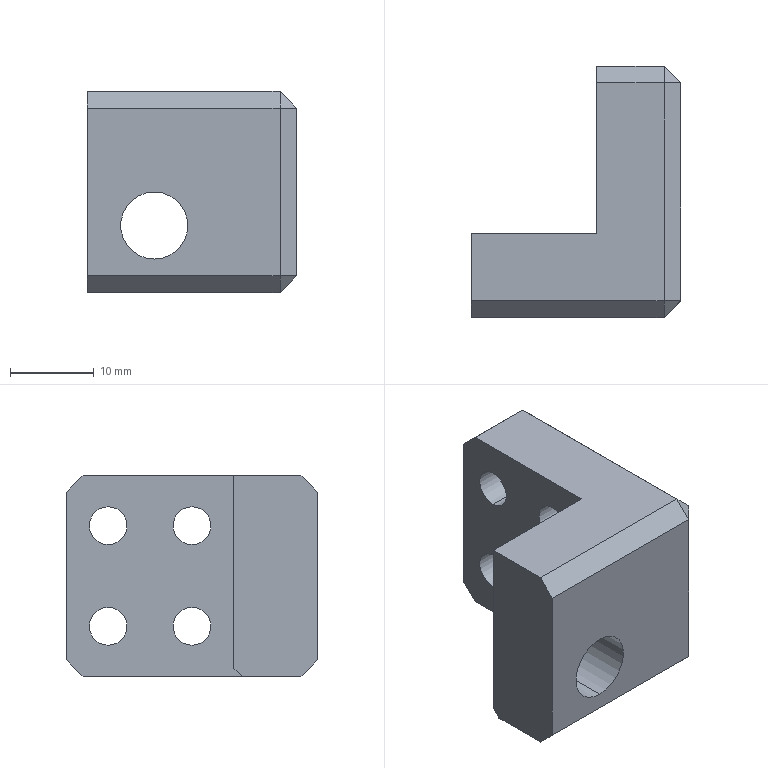Part | NX | features BREP 1 | 1 solid | 45 faces | box 25 x 30 x 24 mm | volume 8772 mm3 | plane 27 | cylinder 18 | commonest cylinder face diameters 8 x10 4.5 x8
STEP:
#1=CARTESIAN_POINT('',(3.971,-310.,10.));
#2=VERTEX_POINT('',#1);
#3=CARTESIAN_POINT('',(3.971,-310.,2.));
#4=VERTEX_POINT('',#3);
#5=CARTESIAN_POINT('',(3.971,-310.,6.));
#6=DIRECTION('',(1.,0.,0.));
#7=DIRECTION('',(0.,0.,-1.));
#8=AXIS2_PLACEMENT_3D('',#5,#6,#7);
#9=CIRCLE('',#8,4.);
#10=EDGE_CURVE('',#2,#4,#9,.T.);
#11=ORIENTED_EDGE('',*,*,#10,.F.);
#12=CARTESIAN_POINT('',(7.971,-310.,10.));
#13=VERTEX_POINT('',#12);
#14=CARTESIAN_POINT('',(7.971,-310.,10.));
#15=DIRECTION('',(1.,0.,0.));
#16=VECTOR('',#15,1000.);
#17=LINE('',#14,#16);
#18=EDGE_CURVE('',#2,#13,#17,.T.);
#19=ORIENTED_EDGE('',*,*,#18,.T.);
#20=CARTESIAN_POINT('',(7.971,-310.,2.));
#21=VERTEX_POINT('',#20);
#22=CARTESIAN_POINT('',(7.971,-310.,6.));
#23=DIRECTION('',(1.,0.,0.));
#24=DIRECTION('',(0.,0.,-1.));
#25=AXIS2_PLACEMENT_3D('',#22,#23,#24);
#26=CIRCLE('',#25,4.);
#27=EDGE_CURVE('',#13,#21,#26,.T.);
#28=ORIENTED_EDGE('',*,*,#27,.T.);
#29=CARTESIAN_POINT('',(7.971,-310.,2.));
#30=DIRECTION('',(1.,0.,0.));
#31=VECTOR('',#30,1000.);
#32=LINE('',#29,#31);
#33=EDGE_CURVE('',#4,#21,#32,.T.);
#34=ORIENTED_EDGE('',*,*,#33,.F.);
#35=EDGE_LOOP('',(#11,#19,#28,#34));
#36=FACE_BOUND('',#35,.T.);
#37=CARTESIAN_POINT('',(7.971,-310.,6.));
#38=DIRECTION('',(1.,0.,0.));
#39=DIRECTION('',(0.,0.,-1.));
#40=AXIS2_PLACEMENT_3D('',#37,#38,#39);
#41=CYLINDRICAL_SURFACE('',#40,4.);
#42=ADVANCED_FACE('',(#36),#41,.F.);
#43=CARTESIAN_POINT('',(-2.029,-310.,8.25));
#44=VERTEX_POINT('',#43);
#45=CARTESIAN_POINT('',(-2.029,-310.,3.75));
#46=VERTEX_POINT('',#45);
#47=CARTESIAN_POINT('',(-2.029,-310.,6.));
#48=DIRECTION('',(1.,0.,0.));
#49=DIRECTION('',(0.,1.,0.));
#50=AXIS2_PLACEMENT_3D('',#47,#48,#49);
#51=CIRCLE('',#50,2.25);
#52=EDGE_CURVE('',#44,#46,#51,.T.);
#53=ORIENTED_EDGE('',*,*,#52,.F.);
#54=CARTESIAN_POINT('',(3.971,-310.,8.25));
#55=VERTEX_POINT('',#54);
#56=CARTESIAN_POINT('',(7.971,-310.,8.25));
#57=DIRECTION('',(1.,0.,0.));
#58=VECTOR('',#57,1000.);
#59=LINE('',#56,#58);
#60=EDGE_CURVE('',#44,#55,#59,.T.);
#61=ORIENTED_EDGE('',*,*,#60,.T.);
#62=CARTESIAN_POINT('',(3.971,-310.,3.75));
#63=VERTEX_POINT('',#62);
#64=CARTESIAN_POINT('',(3.971,-310.,6.));
#65=DIRECTION('',(1.,0.,0.));
#66=DIRECTION('',(0.,0.,-1.));
#67=AXIS2_PLACEMENT_3D('',#64,#65,#66);
#68=CIRCLE('',#67,2.25);
#69=EDGE_CURVE('',#55,#63,#68,.T.);
#70=ORIENTED_EDGE('',*,*,#69,.T.);
#71=CARTESIAN_POINT('',(7.971,-310.,3.75));
#72=DIRECTION('',(1.,0.,0.));
#73=VECTOR('',#72,1000.);
#74=LINE('',#71,#73);
#75=EDGE_CURVE('',#46,#63,#74,.T.);
#76=ORIENTED_EDGE('',*,*,#75,.F.);
#77=EDGE_LOOP('',(#53,#61,#70,#76));
#78=FACE_BOUND('',#77,.T.);
#79=CARTESIAN_POINT('',(7.971,-310.,6.));
#80=DIRECTION('',(1.,0.,0.));
#81=DIRECTION('',(0.,0.,-1.));
#82=AXIS2_PLACEMENT_3D('',#79,#80,#81);
#83=CYLINDRICAL_SURFACE('',#82,2.25);
#84=ADVANCED_FACE('',(#78),#83,.F.);
#85=CARTESIAN_POINT('',(3.971,-320.,10.));
#86=VERTEX_POINT('',#85);
#87=CARTESIAN_POINT('',(3.971,-320.,2.));
#88=VERTEX_POINT('',#87);
#89=CARTESIAN_POINT('',(3.971,-320.,6.));
#90=DIRECTION('',(1.,0.,0.));
#91=DIRECTION('',(0.,0.,-1.));
#92=AXIS2_PLACEMENT_3D('',#89,#90,#91);
#93=CIRCLE('',#92,4.);
#94=EDGE_CURVE('',#86,#88,#93,.T.);
#95=ORIENTED_EDGE('',*,*,#94,.F.);
#96=CARTESIAN_POINT('',(7.971,-320.,10.));
#97=VERTEX_POINT('',#96);
#98=CARTESIAN_POINT('',(7.971,-320.,10.));
#99=DIRECTION('',(1.,0.,0.));
#100=VECTOR('',#99,1000.);
#101=LINE('',#98,#100);
#102=EDGE_CURVE('',#86,#97,#101,.T.);
#103=ORIENTED_EDGE('',*,*,#102,.T.);
#104=CARTESIAN_POINT('',(7.971,-320.,2.));
#105=VERTEX_POINT('',#104);
#106=CARTESIAN_POINT('',(7.971,-320.,6.));
#107=DIRECTION('',(1.,0.,0.));
#108=DIRECTION('',(0.,0.,-1.));
#109=AXIS2_PLACEMENT_3D('',#106,#107,#108);
#110=CIRCLE('',#109,4.);
#111=EDGE_CURVE('',#97,#105,#110,.T.);
#112=ORIENTED_EDGE('',*,*,#111,.T.);
#113=CARTESIAN_POINT('',(7.971,-320.,2.));
#114=DIRECTION('',(1.,0.,0.));
#115=VECTOR('',#114,1000.);
#116=LINE('',#113,#115);
#117=EDGE_CURVE('',#88,#105,#116,.T.);
#118=ORIENTED_EDGE('',*,*,#117,.F.);
#119=EDGE_LOOP('',(#95,#103,#112,#118));
#120=FACE_BOUND('',#119,.T.);
#121=CARTESIAN_POINT('',(7.971,-320.,6.));
#122=DIRECTION('',(1.,0.,0.));
#123=DIRECTION('',(0.,0.,-1.));
#124=AXIS2_PLACEMENT_3D('',#121,#122,#123);
#125=CYLINDRICAL_SURFACE('',#124,4.);
#126=ADVANCED_FACE('',(#120),#125,.F.);
#127=CARTESIAN_POINT('',(-2.029,-320.,8.25));
#128=VERTEX_POINT('',#127);
#129=CARTESIAN_POINT('',(-2.029,-320.,3.75));
#130=VERTEX_POINT('',#129);
#131=CARTESIAN_POINT('',(-2.029,-320.,6.));
#132=DIRECTION('',(1.,0.,0.));
#133=DIRECTION('',(0.,1.,0.));
#134=AXIS2_PLACEMENT_3D('',#131,#132,#133);
#135=CIRCLE('',#134,2.25);
#136=EDGE_CURVE('',#128,#130,#135,.T.);
#137=ORIENTED_EDGE('',*,*,#136,.F.);
#138=CARTESIAN_POINT('',(3.971,-320.,8.25));
#139=VERTEX_POINT('',#138);
#140=CARTESIAN_POINT('',(7.971,-320.,8.25));
#141=DIRECTION('',(1.,0.,0.));
#142=VECTOR('',#141,1000.);
#143=LINE('',#140,#142);
#144=EDGE_CURVE('',#128,#139,#143,.T.);
#145=ORIENTED_EDGE('',*,*,#144,.T.);
#146=CARTESIAN_POINT('',(3.971,-320.,3.75));
#147=VERTEX_POINT('',#146);
#148=CARTESIAN_POINT('',(3.971,-320.,6.));
#149=DIRECTION('',(1.,0.,0.));
#150=DIRECTION('',(0.,0.,-1.));
#151=AXIS2_PLACEMENT_3D('',#148,#149,#150);
#152=CIRCLE('',#151,2.25);
#153=EDGE_CURVE('',#139,#147,#152,.T.);
#154=ORIENTED_EDGE('',*,*,#153,.T.);
#155=CARTESIAN_POINT('',(7.971,-320.,3.75));
#156=DIRECTION('',(1.,0.,0.));
#157=VECTOR('',#156,1000.);
#158=LINE('',#155,#157);
#159=EDGE_CURVE('',#130,#147,#158,.T.);
#160=ORIENTED_EDGE('',*,*,#159,.F.);
#161=EDGE_LOOP('',(#137,#145,#154,#160));
#162=FACE_BOUND('',#161,.T.);
#163=CARTESIAN_POINT('',(7.971,-320.,6.));
#164=DIRECTION('',(1.,0.,0.));
#165=DIRECTION('',(0.,0.,-1.));
#166=AXIS2_PLACEMENT_3D('',#163,#164,#165);
#167=CYLINDRICAL_SURFACE('',#166,2.25);
#168=ADVANCED_FACE('',(#162),#167,.F.);
#169=CARTESIAN_POINT('',(3.971,-310.,22.));
#170=VERTEX_POINT('',#169);
#171=CARTESIAN_POINT('',(3.971,-310.,14.));
#172=VERTEX_POINT('',#171);
#173=CARTESIAN_POINT('',(3.971,-310.,18.));
#174=DIRECTION('',(1.,0.,0.));
#175=DIRECTION('',(0.,0.,-1.));
#176=AXIS2_PLACEMENT_3D('',#173,#174,#175);
#177=CIRCLE('',#176,4.);
#178=EDGE_CURVE('',#170,#172,#177,.T.);
#179=ORIENTED_EDGE('',*,*,#178,.F.);
#180=CARTESIAN_POINT('',(7.971,-310.,22.));
#181=VERTEX_POINT('',#180);
#182=CARTESIAN_POINT('',(7.971,-310.,22.));
#183=DIRECTION('',(1.,0.,0.));
#184=VECTOR('',#183,1000.);
#185=LINE('',#182,#184);
#186=EDGE_CURVE('',#170,#181,#185,.T.);
#187=ORIENTED_EDGE('',*,*,#186,.T.);
#188=CARTESIAN_POINT('',(7.971,-310.,14.));
#189=VERTEX_POINT('',#188);
#190=CARTESIAN_POINT('',(7.971,-310.,18.));
#191=DIRECTION('',(1.,0.,0.));
#192=DIRECTION('',(0.,0.,-1.));
#193=AXIS2_PLACEMENT_3D('',#190,#191,#192);
#194=CIRCLE('',#193,4.);
#195=EDGE_CURVE('',#181,#189,#194,.T.);
#196=ORIENTED_EDGE('',*,*,#195,.T.);
#197=CARTESIAN_POINT('',(7.971,-310.,14.));
#198=DIRECTION('',(1.,0.,0.));
#199=VECTOR('',#198,1000.);
#200=LINE('',#197,#199);
#201=EDGE_CURVE('',#172,#189,#200,.T.);
#202=ORIENTED_EDGE('',*,*,#201,.F.);
#203=EDGE_LOOP('',(#179,#187,#196,#202));
#204=FACE_BOUND('',#203,.T.);
#205=CARTESIAN_POINT('',(7.971,-310.,18.));
#206=DIRECTION('',(1.,0.,0.));
#207=DIRECTION('',(0.,0.,-1.));
#208=AXIS2_PLACEMENT_3D('',#205,#206,#207);
#209=CYLINDRICAL_SURFACE('',#208,4.);
#210=ADVANCED_FACE('',(#204),#209,.F.);
#211=CARTESIAN_POINT('',(-2.029,-310.,20.25));
#212=VERTEX_POINT('',#211);
#213=CARTESIAN_POINT('',(-2.029,-310.,15.75));
#214=VERTEX_POINT('',#213);
#215=CARTESIAN_POINT('',(-2.029,-310.,18.));
#216=DIRECTION('',(1.,0.,0.));
#217=DIRECTION('',(0.,1.,0.));
#218=AXIS2_PLACEMENT_3D('',#215,#216,#217);
#219=CIRCLE('',#218,2.25);
#220=EDGE_CURVE('',#212,#214,#219,.T.);
#221=ORIENTED_EDGE('',*,*,#220,.F.);
#222=CARTESIAN_POINT('',(3.971,-310.,20.25));
#223=VERTEX_POINT('',#222);
#224=CARTESIAN_POINT('',(7.971,-310.,20.25));
#225=DIRECTION('',(1.,0.,0.));
#226=VECTOR('',#225,1000.);
#227=LINE('',#224,#226);
#228=EDGE_CURVE('',#212,#223,#227,.T.);
#229=ORIENTED_EDGE('',*,*,#228,.T.);
#230=CARTESIAN_POINT('',(3.971,-310.,15.75));
#231=VERTEX_POINT('',#230);
#232=CARTESIAN_POINT('',(3.971,-310.,18.));
#233=DIRECTION('',(1.,0.,0.));
#234=DIRECTION('',(0.,0.,-1.));
#235=AXIS2_PLACEMENT_3D('',#232,#233,#234);
#236=CIRCLE('',#235,2.25);
#237=EDGE_CURVE('',#223,#231,#236,.T.);
#238=ORIENTED_EDGE('',*,*,#237,.T.);
#239=CARTESIAN_POINT('',(7.971,-310.,15.75));
#240=DIRECTION('',(1.,0.,0.));
#241=VECTOR('',#240,1000.);
#242=LINE('',#239,#241);
#243=EDGE_CURVE('',#214,#231,#242,.T.);
#244=ORIENTED_EDGE('',*,*,#243,.F.);
#245=EDGE_LOOP('',(#221,#229,#238,#244));
#246=FACE_BOUND('',#245,.T.);
#247=CARTESIAN_POINT('',(7.971,-310.,18.));
#248=DIRECTION('',(1.,0.,0.));
#249=DIRECTION('',(0.,0.,-1.));
#250=AXIS2_PLACEMENT_3D('',#247,#248,#249);
#251=CYLINDRICAL_SURFACE('',#250,2.25);
#252=ADVANCED_FACE('',(#246),#251,.F.);
#253=CARTESIAN_POINT('',(3.971,-320.,22.));
#254=VERTEX_POINT('',#253);
#255=CARTESIAN_POINT('',(3.971,-320.,14.));
#256=VERTEX_POINT('',#255);
#257=CARTESIAN_POINT('',(3.971,-320.,18.));
#258=DIRECTION('',(1.,0.,0.));
#259=DIRECTION('',(0.,0.,-1.));
#260=AXIS2_PLACEMENT_3D('',#257,#258,#259);
#261=CIRCLE('',#260,4.);
#262=EDGE_CURVE('',#254,#256,#261,.T.);
#263=ORIENTED_EDGE('',*,*,#262,.F.);
#264=CARTESIAN_POINT('',(7.971,-320.,22.));
#265=VERTEX_POINT('',#264);
#266=CARTESIAN_POINT('',(7.971,-320.,22.));
#267=DIRECTION('',(1.,0.,0.));
#268=VECTOR('',#267,1000.);
#269=LINE('',#266,#268);
#270=EDGE_CURVE('',#254,#265,#269,.T.);
#271=ORIENTED_EDGE('',*,*,#270,.T.);
#272=CARTESIAN_POINT('',(7.971,-320.,14.));
#273=VERTEX_POINT('',#272);
#274=CARTESIAN_POINT('',(7.971,-320.,18.));
#275=DIRECTION('',(1.,0.,0.));
#276=DIRECTION('',(0.,0.,-1.));
#277=AXIS2_PLACEMENT_3D('',#274,#275,#276);
#278=CIRCLE('',#277,4.);
#279=EDGE_CURVE('',#265,#273,#278,.T.);
#280=ORIENTED_EDGE('',*,*,#279,.T.);
#281=CARTESIAN_POINT('',(7.971,-320.,14.));
#282=DIRECTION('',(1.,0.,0.));
#283=VECTOR('',#282,1000.);
#284=LINE('',#281,#283);
#285=EDGE_CURVE('',#256,#273,#284,.T.);
#286=ORIENTED_EDGE('',*,*,#285,.F.);
#287=EDGE_LOOP('',(#263,#271,#280,#286));
#288=FACE_BOUND('',#287,.T.);
#289=CARTESIAN_POINT('',(7.971,-320.,18.));
#290=DIRECTION('',(1.,0.,0.));
#291=DIRECTION('',(0.,0.,-1.));
#292=AXIS2_PLACEMENT_3D('',#289,#290,#291);
#293=CYLINDRICAL_SURFACE('',#292,4.);
#294=ADVANCED_FACE('',(#288),#293,.F.);
#295=CARTESIAN_POINT('',(-2.029,-320.,20.25));
#296=VERTEX_POINT('',#295);
#297=CARTESIAN_POINT('',(-2.029,-320.,15.75));
#298=VERTEX_POINT('',#297);
#299=CARTESIAN_POINT('',(-2.029,-320.,18.));
#300=DIRECTION('',(1.,0.,0.));
#301=DIRECTION('',(0.,1.,0.));
#302=AXIS2_PLACEMENT_3D('',#299,#300,#301);
#303=CIRCLE('',#302,2.25);
#304=EDGE_CURVE('',#296,#298,#303,.T.);
#305=ORIENTED_EDGE('',*,*,#304,.F.);
#306=CARTESIAN_POINT('',(3.971,-320.,20.25));
#307=VERTEX_POINT('',#306);
#308=CARTESIAN_POINT('',(7.971,-320.,20.25));
#309=DIRECTION('',(1.,0.,0.));
#310=VECTOR('',#309,1000.);
#311=LINE('',#308,#310);
#312=EDGE_CURVE('',#296,#307,#311,.T.);
#313=ORIENTED_EDGE('',*,*,#312,.T.);
#314=CARTESIAN_POINT('',(3.971,-320.,15.75));
#315=VERTEX_POINT('',#314);
#316=CARTESIAN_POINT('',(3.971,-320.,18.));
#317=DIRECTION('',(1.,0.,0.));
#318=DIRECTION('',(0.,0.,-1.));
#319=AXIS2_PLACEMENT_3D('',#316,#317,#318);
#320=CIRCLE('',#319,2.25);
#321=EDGE_CURVE('',#307,#315,#320,.T.);
#322=ORIENTED_EDGE('',*,*,#321,.T.);
#323=CARTESIAN_POINT('',(7.971,-320.,15.75));
#324=DIRECTION('',(1.,0.,0.));
#325=VECTOR('',#324,1000.);
#326=LINE('',#323,#325);
#327=EDGE_CURVE('',#298,#315,#326,.T.);
#328=ORIENTED_EDGE('',*,*,#327,.F.);
#329=EDGE_LOOP('',(#305,#313,#322,#328));
#330=FACE_BOUND('',#329,.T.);
#331=CARTESIAN_POINT('',(7.971,-320.,18.));
#332=DIRECTION('',(1.,0.,0.));
#333=DIRECTION('',(0.,0.,-1.));
#334=AXIS2_PLACEMENT_3D('',#331,#332,#333);
#335=CYLINDRICAL_SURFACE('',#334,2.25);
#336=ADVANCED_FACE('',(#330),#335,.F.);
#337=CARTESIAN_POINT('',(-9.029,-325.,12.));
#338=VERTEX_POINT('',#337);
#339=CARTESIAN_POINT('',(-9.029,-325.,4.));
#340=VERTEX_POINT('',#339);
#341=CARTESIAN_POINT('',(-9.029,-325.,8.));
#342=DIRECTION('',(0.,-1.,0.));
#343=DIRECTION('',(0.,0.,-1.));
#344=AXIS2_PLACEMENT_3D('',#341,#342,#343);
#345=CIRCLE('',#344,4.);
#346=EDGE_CURVE('',#338,#340,#345,.T.);
#347=ORIENTED_EDGE('',*,*,#346,.F.);
#348=CARTESIAN_POINT('',(-9.029,-335.,12.));
#349=VERTEX_POINT('',#348);
#350=CARTESIAN_POINT('',(-9.029,-305.,12.));
#351=DIRECTION('',(0.,-1.,0.));
#352=VECTOR('',#351,1000.);
#353=LINE('',#350,#352);
#354=EDGE_CURVE('',#338,#349,#353,.T.);
#355=ORIENTED_EDGE('',*,*,#354,.T.);
#356=CARTESIAN_POINT('',(-9.029,-335.,4.));
#357=VERTEX_POINT('',#356);
#358=CARTESIAN_POINT('',(-9.029,-335.,8.));
#359=DIRECTION('',(0.,-1.,0.));
#360=DIRECTION('',(0.,0.,-1.));
#361=AXIS2_PLACEMENT_3D('',#358,#359,#360);
#362=CIRCLE('',#361,4.);
#363=EDGE_CURVE('',#349,#357,#362,.T.);
#364=ORIENTED_EDGE('',*,*,#363,.T.);
#365=CARTESIAN_POINT('',(-9.029,-305.,4.));
#366=DIRECTION('',(0.,-1.,0.));
#367=VECTOR('',#366,1000.);
#368=LINE('',#365,#367);
#369=EDGE_CURVE('',#340,#357,#368,.T.);
#370=ORIENTED_EDGE('',*,*,#369,.F.);
#371=EDGE_LOOP('',(#347,#355,#364,#370));
#372=FACE_BOUND('',#371,.T.);
#373=CARTESIAN_POINT('',(-9.029,-305.,8.));
#374=DIRECTION('',(0.,-1.,0.));
#375=DIRECTION('',(0.,0.,-1.));
#376=AXIS2_PLACEMENT_3D('',#373,#374,#375);
#377=CYLINDRICAL_SURFACE('',#376,4.);
#378=ADVANCED_FACE('',(#372),#377,.F.);
#379=CARTESIAN_POINT('',(7.971,-307.,8.646));
#380=VERTEX_POINT('',#379);
#381=CARTESIAN_POINT('',(7.971,-310.,6.));
#382=DIRECTION('',(1.,0.,0.));
#383=DIRECTION('',(0.,0.,-1.));
#384=AXIS2_PLACEMENT_3D('',#381,#382,#383);
#385=CIRCLE('',#384,4.);
#386=EDGE_CURVE('',#380,#13,#385,.T.);
#387=ORIENTED_EDGE('',*,*,#386,.F.);
#388=CARTESIAN_POINT('',(7.971,-307.,15.354));
#389=VERTEX_POINT('',#388);
#390=CARTESIAN_POINT('',(7.971,-307.,24.));
#391=DIRECTION('',(0.,0.,1.));
#392=VECTOR('',#391,1000.);
#393=LINE('',#390,#392);
#394=EDGE_CURVE('',#380,#389,#393,.T.);
#395=ORIENTED_EDGE('',*,*,#394,.T.);
#396=CARTESIAN_POINT('',(7.971,-310.,18.));
#397=DIRECTION('',(1.,0.,0.));
#398=DIRECTION('',(0.,0.,-1.));
#399=AXIS2_PLACEMENT_3D('',#396,#397,#398);
#400=CIRCLE('',#399,4.);
#401=EDGE_CURVE('',#189,#389,#400,.T.);
#402=ORIENTED_EDGE('',*,*,#401,.F.);
#403=ORIENTED_EDGE('',*,*,#195,.F.);
#404=CARTESIAN_POINT('',(7.971,-305.,22.));
#405=DIRECTION('',(0.,-1.,0.));
#406=VECTOR('',#405,1000.);
#407=LINE('',#404,#406);
#408=EDGE_CURVE('',#181,#265,#407,.T.);
#409=ORIENTED_EDGE('',*,*,#408,.T.);
#410=CARTESIAN_POINT('',(7.971,-320.,18.));
#411=DIRECTION('',(1.,0.,0.));
#412=DIRECTION('',(0.,0.,-1.));
#413=AXIS2_PLACEMENT_3D('',#410,#411,#412);
#414=CIRCLE('',#413,4.);
#415=EDGE_CURVE('',#273,#265,#414,.T.);
#416=ORIENTED_EDGE('',*,*,#415,.F.);
#417=ORIENTED_EDGE('',*,*,#279,.F.);
#418=CARTESIAN_POINT('',(7.971,-333.,22.));
#419=VERTEX_POINT('',#418);
#420=CARTESIAN_POINT('',(7.971,-305.,22.));
#421=DIRECTION('',(0.,-1.,0.));
#422=VECTOR('',#421,1000.);
#423=LINE('',#420,#422);
#424=EDGE_CURVE('',#265,#419,#423,.T.);
#425=ORIENTED_EDGE('',*,*,#424,.T.);
#426=CARTESIAN_POINT('',(7.971,-333.,2.));
#427=VERTEX_POINT('',#426);
#428=CARTESIAN_POINT('',(7.971,-333.,24.));
#429=DIRECTION('',(0.,0.,-1.));
#430=VECTOR('',#429,1000.);
#431=LINE('',#428,#430);
#432=EDGE_CURVE('',#419,#427,#431,.T.);
#433=ORIENTED_EDGE('',*,*,#432,.T.);
#434=CARTESIAN_POINT('',(7.971,-305.,2.));
#435=DIRECTION('',(0.,1.,0.));
#436=VECTOR('',#435,1000.);
#437=LINE('',#434,#436);
#438=EDGE_CURVE('',#427,#105,#437,.T.);
#439=ORIENTED_EDGE('',*,*,#438,.T.);
#440=ORIENTED_EDGE('',*,*,#111,.F.);
#441=CARTESIAN_POINT('',(7.971,-320.,6.));
#442=DIRECTION('',(1.,0.,0.));
#443=DIRECTION('',(0.,0.,-1.));
#444=AXIS2_PLACEMENT_3D('',#441,#442,#443);
#445=CIRCLE('',#444,4.);
#446=EDGE_CURVE('',#105,#97,#445,.T.);
#447=ORIENTED_EDGE('',*,*,#446,.F.);
#448=CARTESIAN_POINT('',(7.971,-305.,2.));
#449=DIRECTION('',(0.,1.,0.));
#450=VECTOR('',#449,1000.);
#451=LINE('',#448,#450);
#452=EDGE_CURVE('',#105,#21,#451,.T.);
#453=ORIENTED_EDGE('',*,*,#452,.T.);
#454=ORIENTED_EDGE('',*,*,#27,.F.);
#455=EDGE_LOOP('',(#387,#395,#402,#403,#409,#416,#417,#425,#433,#439,#440,#447,#453,#454));
#456=FACE_BOUND('',#455,.T.);
#457=CARTESIAN_POINT('',(7.971,-305.,24.));
#458=DIRECTION('',(-1.,0.,0.));
#459=DIRECTION('',(0.,1.,0.));
#460=AXIS2_PLACEMENT_3D('',#457,#458,#459);
#461=PLANE('',#460);
#462=ADVANCED_FACE('',(#456),#461,.F.);
#463=CARTESIAN_POINT('',(7.971,-307.,2.));
#464=VERTEX_POINT('',#463);
#465=CARTESIAN_POINT('',(7.971,-305.,2.));
#466=DIRECTION('',(0.,1.,0.));
#467=VECTOR('',#466,1000.);
#468=LINE('',#465,#467);
#469=EDGE_CURVE('',#21,#464,#468,.T.);
#470=ORIENTED_EDGE('',*,*,#469,.T.);
#471=CARTESIAN_POINT('',(7.971,-307.,3.354));
#472=VERTEX_POINT('',#471);
#473=CARTESIAN_POINT('',(7.971,-307.,24.));
#474=DIRECTION('',(0.,0.,1.));
#475=VECTOR('',#474,1000.);
#476=LINE('',#473,#475);
#477=EDGE_CURVE('',#464,#472,#476,.T.);
#478=ORIENTED_EDGE('',*,*,#477,.T.);
#479=CARTESIAN_POINT('',(7.971,-310.,6.));
#480=DIRECTION('',(1.,0.,0.));
#481=DIRECTION('',(0.,0.,-1.));
#482=AXIS2_PLACEMENT_3D('',#479,#480,#481);
#483=CIRCLE('',#482,4.);
#484=EDGE_CURVE('',#21,#472,#483,.T.);
#485=ORIENTED_EDGE('',*,*,#484,.F.);
#486=EDGE_LOOP('',(#470,#478,#485));
#487=FACE_BOUND('',#486,.T.);
#488=CARTESIAN_POINT('',(7.971,-305.,24.));
#489=DIRECTION('',(-1.,0.,0.));
#490=DIRECTION('',(0.,1.,0.));
#491=AXIS2_PLACEMENT_3D('',#488,#489,#490);
#492=PLANE('',#491);
#493=ADVANCED_FACE('',(#487),#492,.F.);
#494=CARTESIAN_POINT('',(-2.029,-305.,22.));
#495=VERTEX_POINT('',#494);
#496=CARTESIAN_POINT('',(-2.029,-305.,2.));
#497=VERTEX_POINT('',#496);
#498=CARTESIAN_POINT('',(-2.029,-305.,24.));
#499=DIRECTION('',(0.,0.,-1.));
#500=VECTOR('',#499,1000.);
#501=LINE('',#498,#500);
#502=EDGE_CURVE('',#495,#497,#501,.T.);
#503=ORIENTED_EDGE('',*,*,#502,.T.);
#504=CARTESIAN_POINT('',(-2.029,-307.,0.));
#505=VERTEX_POINT('',#504);
#506=CARTESIAN_POINT('',(-2.029,-305.,2.));
#507=DIRECTION('',(0.,-0.7071,-0.7071));
#508=VECTOR('',#507,1000.);
#509=LINE('',#506,#508);
#510=EDGE_CURVE('',#497,#505,#509,.T.);
#511=ORIENTED_EDGE('',*,*,#510,.T.);
#512=CARTESIAN_POINT('',(-2.029,-326.,0.));
#513=VERTEX_POINT('',#512);
#514=CARTESIAN_POINT('',(-2.029,-305.,0.));
#515=DIRECTION('',(0.,-1.,0.));
#516=VECTOR('',#515,1000.);
#517=LINE('',#514,#516);
#518=EDGE_CURVE('',#505,#513,#517,.T.);
#519=ORIENTED_EDGE('',*,*,#518,.T.);
#520=CARTESIAN_POINT('',(-2.029,-325.,1.));
#521=VERTEX_POINT('',#520);
#522=CARTESIAN_POINT('',(-2.029,-303.5,22.5));
#523=DIRECTION('',(0.,0.7071,0.7071));
#524=VECTOR('',#523,1000.);
#525=LINE('',#522,#524);
#526=EDGE_CURVE('',#513,#521,#525,.T.);
#527=ORIENTED_EDGE('',*,*,#526,.T.);
#528=CARTESIAN_POINT('',(-2.029,-325.,24.));
#529=VERTEX_POINT('',#528);
#530=CARTESIAN_POINT('',(-2.029,-325.,24.));
#531=DIRECTION('',(0.,0.,-1.));
#532=VECTOR('',#531,1000.);
#533=LINE('',#530,#532);
#534=EDGE_CURVE('',#529,#521,#533,.T.);
#535=ORIENTED_EDGE('',*,*,#534,.F.);
#536=CARTESIAN_POINT('',(-2.029,-307.,24.));
#537=VERTEX_POINT('',#536);
#538=CARTESIAN_POINT('',(-2.029,-305.,24.));
#539=DIRECTION('',(0.,-1.,0.));
#540=VECTOR('',#539,1000.);
#541=LINE('',#538,#540);
#542=EDGE_CURVE('',#537,#529,#541,.T.);
#543=ORIENTED_EDGE('',*,*,#542,.F.);
#544=CARTESIAN_POINT('',(-2.029,-307.,24.));
#545=DIRECTION('',(0.,0.7071,-0.7071));
#546=VECTOR('',#545,1000.);
#547=LINE('',#544,#546);
#548=EDGE_CURVE('',#537,#495,#547,.T.);
#549=ORIENTED_EDGE('',*,*,#548,.T.);
#550=EDGE_LOOP('',(#503,#511,#519,#527,#535,#543,#549));
#551=FACE_BOUND('',#550,.T.);
#552=CARTESIAN_POINT('',(-2.029,-310.,6.));
#553=DIRECTION('',(1.,0.,0.));
#554=DIRECTION('',(0.,1.,0.));
#555=AXIS2_PLACEMENT_3D('',#552,#553,#554);
#556=CIRCLE('',#555,2.25);
#557=EDGE_CURVE('',#46,#44,#556,.T.);
#558=ORIENTED_EDGE('',*,*,#557,.T.);
#559=ORIENTED_EDGE('',*,*,#52,.T.);
#560=EDGE_LOOP('',(#558,#559));
#561=FACE_BOUND('',#560,.T.);
#562=CARTESIAN_POINT('',(-2.029,-320.,6.));
#563=DIRECTION('',(1.,0.,0.));
#564=DIRECTION('',(0.,1.,0.));
#565=AXIS2_PLACEMENT_3D('',#562,#563,#564);
#566=CIRCLE('',#565,2.25);
#567=EDGE_CURVE('',#130,#128,#566,.T.);
#568=ORIENTED_EDGE('',*,*,#567,.T.);
#569=ORIENTED_EDGE('',*,*,#136,.T.);
#570=EDGE_LOOP('',(#568,#569));
#571=FACE_BOUND('',#570,.T.);
#572=CARTESIAN_POINT('',(-2.029,-310.,18.));
#573=DIRECTION('',(1.,0.,0.));
#574=DIRECTION('',(0.,1.,0.));
#575=AXIS2_PLACEMENT_3D('',#572,#573,#574);
#576=CIRCLE('',#575,2.25);
#577=EDGE_CURVE('',#214,#212,#576,.T.);
#578=ORIENTED_EDGE('',*,*,#577,.T.);
#579=ORIENTED_EDGE('',*,*,#220,.T.);
#580=EDGE_LOOP('',(#578,#579));
#581=FACE_BOUND('',#580,.T.);
#582=CARTESIAN_POINT('',(-2.029,-320.,18.));
#583=DIRECTION('',(1.,0.,0.));
#584=DIRECTION('',(0.,1.,0.));
#585=AXIS2_PLACEMENT_3D('',#582,#583,#584);
#586=CIRCLE('',#585,2.25);
#587=EDGE_CURVE('',#298,#296,#586,.T.);
#588=ORIENTED_EDGE('',*,*,#587,.T.);
#589=ORIENTED_EDGE('',*,*,#304,.T.);
#590=EDGE_LOOP('',(#588,#589));
#591=FACE_BOUND('',#590,.T.);
#592=CARTESIAN_POINT('',(-2.029,-305.,24.));
#593=DIRECTION('',(1.,0.,0.));
#594=DIRECTION('',(0.,1.,0.));
#595=AXIS2_PLACEMENT_3D('',#592,#593,#594);
#596=PLANE('',#595);
#597=ADVANCED_FACE('',(#551,#561,#571,#581,#591),#596,.F.);
#598=ORIENTED_EDGE('',*,*,#534,.T.);
#599=CARTESIAN_POINT('',(-17.029,-325.,1.));
#600=VERTEX_POINT('',#599);
#601=CARTESIAN_POINT('',(-17.029,-325.,1.));
#602=DIRECTION('',(-1.,0.,0.));
#603=VECTOR('',#602,1000.);
#604=LINE('',#601,#603);
#605=EDGE_CURVE('',#521,#600,#604,.T.);
#606=ORIENTED_EDGE('',*,*,#605,.T.);
#607=CARTESIAN_POINT('',(-17.029,-325.,24.));
#608=VERTEX_POINT('',#607);
#609=CARTESIAN_POINT('',(-17.029,-325.,24.));
#610=DIRECTION('',(0.,0.,-1.));
#611=VECTOR('',#610,1000.);
#612=LINE('',#609,#611);
#613=EDGE_CURVE('',#608,#600,#612,.T.);
#614=ORIENTED_EDGE('',*,*,#613,.F.);
#615=CARTESIAN_POINT('',(-2.029,-325.,24.));
#616=DIRECTION('',(-1.,0.,0.));
#617=VECTOR('',#616,1000.);
#618=LINE('',#615,#617);
#619=EDGE_CURVE('',#529,#608,#618,.T.);
#620=ORIENTED_EDGE('',*,*,#619,.F.);
#621=EDGE_LOOP('',(#598,#606,#614,#620));
#622=FACE_BOUND('',#621,.T.);
#623=CARTESIAN_POINT('',(-9.029,-325.,8.));
#624=DIRECTION('',(0.,-1.,0.));
#625=DIRECTION('',(0.,0.,-1.));
#626=AXIS2_PLACEMENT_3D('',#623,#624,#625);
#627=CIRCLE('',#626,4.);
#628=EDGE_CURVE('',#340,#338,#627,.T.);
#629=ORIENTED_EDGE('',*,*,#628,.T.);
#630=ORIENTED_EDGE('',*,*,#346,.T.);
#631=EDGE_LOOP('',(#629,#630));
#632=FACE_BOUND('',#631,.T.);
#633=CARTESIAN_POINT('',(-2.029,-325.,24.));
#634=DIRECTION('',(0.,-1.,0.));
#635=DIRECTION('',(0.,0.,-1.));
#636=AXIS2_PLACEMENT_3D('',#633,#634,#635);
#637=PLANE('',#636);
#638=ADVANCED_FACE('',(#622,#632),#637,.F.);
#639=ORIENTED_EDGE('',*,*,#613,.T.);
#640=CARTESIAN_POINT('',(-17.029,-326.,0.));
#641=VERTEX_POINT('',#640);
#642=CARTESIAN_POINT('',(-17.029,-325.,1.));
#643=DIRECTION('',(0.,-0.7071,-0.7071));
#644=VECTOR('',#643,1000.);
#645=LINE('',#642,#644);
#646=EDGE_CURVE('',#600,#641,#645,.T.);
#647=ORIENTED_EDGE('',*,*,#646,.T.);
#648=CARTESIAN_POINT('',(-17.029,-333.,0.));
#649=VERTEX_POINT('',#648);
#650=CARTESIAN_POINT('',(-17.029,-325.,0.));
#651=DIRECTION('',(0.,-1.,0.));
#652=VECTOR('',#651,1000.);
#653=LINE('',#650,#652);
#654=EDGE_CURVE('',#641,#649,#653,.T.);
#655=ORIENTED_EDGE('',*,*,#654,.T.);
#656=CARTESIAN_POINT('',(-17.029,-335.,2.));
#657=VERTEX_POINT('',#656);
#658=CARTESIAN_POINT('',(-17.029,-335.,2.));
#659=DIRECTION('',(0.,-0.7071,0.7071));
#660=VECTOR('',#659,1000.);
#661=LINE('',#658,#660);
#662=EDGE_CURVE('',#649,#657,#661,.T.);
#663=ORIENTED_EDGE('',*,*,#662,.T.);
#664=CARTESIAN_POINT('',(-17.029,-335.,22.));
#665=VERTEX_POINT('',#664);
#666=CARTESIAN_POINT('',(-17.029,-335.,24.));
#667=DIRECTION('',(0.,0.,-1.));
#668=VECTOR('',#667,1000.);
#669=LINE('',#666,#668);
#670=EDGE_CURVE('',#665,#657,#669,.T.);
#671=ORIENTED_EDGE('',*,*,#670,.F.);
#672=CARTESIAN_POINT('',(-17.029,-333.,24.));
#673=VERTEX_POINT('',#672);
#674=CARTESIAN_POINT('',(-17.029,-333.,24.));
#675=DIRECTION('',(0.,0.7071,0.7071));
#676=VECTOR('',#675,1000.);
#677=LINE('',#674,#676);
#678=EDGE_CURVE('',#665,#673,#677,.T.);
#679=ORIENTED_EDGE('',*,*,#678,.T.);
#680=CARTESIAN_POINT('',(-17.029,-325.,24.));
#681=DIRECTION('',(0.,-1.,0.));
#682=VECTOR('',#681,1000.);
#683=LINE('',#680,#682);
#684=EDGE_CURVE('',#608,#673,#683,.T.);
#685=ORIENTED_EDGE('',*,*,#684,.F.);
#686=EDGE_LOOP('',(#639,#647,#655,#663,#671,#679,#685));
#687=FACE_BOUND('',#686,.T.);
#688=CARTESIAN_POINT('',(-17.029,-325.,24.));
#689=DIRECTION('',(1.,0.,0.));
#690=DIRECTION('',(0.,1.,0.));
#691=AXIS2_PLACEMENT_3D('',#688,#689,#690);
#692=PLANE('',#691);
#693=ADVANCED_FACE('',(#687),#692,.F.);
#694=ORIENTED_EDGE('',*,*,#670,.T.);
#695=CARTESIAN_POINT('',(5.971,-335.,2.));
#696=VERTEX_POINT('',#695);
#697=CARTESIAN_POINT('',(7.971,-335.,2.));
#698=DIRECTION('',(1.,0.,0.));
#699=VECTOR('',#698,1000.);
#700=LINE('',#697,#699);
#701=EDGE_CURVE('',#657,#696,#700,.T.);
#702=ORIENTED_EDGE('',*,*,#701,.T.);
#703=CARTESIAN_POINT('',(5.971,-335.,22.));
#704=VERTEX_POINT('',#703);
#705=CARTESIAN_POINT('',(5.971,-335.,24.));
#706=DIRECTION('',(0.,0.,1.));
#707=VECTOR('',#706,1000.);
#708=LINE('',#705,#707);
#709=EDGE_CURVE('',#696,#704,#708,.T.);
#710=ORIENTED_EDGE('',*,*,#709,.T.);
#711=CARTESIAN_POINT('',(7.971,-335.,22.));
#712=DIRECTION('',(-1.,0.,0.));
#713=VECTOR('',#712,1000.);
#714=LINE('',#711,#713);
#715=EDGE_CURVE('',#704,#665,#714,.T.);
#716=ORIENTED_EDGE('',*,*,#715,.T.);
#717=EDGE_LOOP('',(#694,#702,#710,#716));
#718=FACE_BOUND('',#717,.T.);
#719=CARTESIAN_POINT('',(-9.029,-335.,8.));
#720=DIRECTION('',(0.,-1.,0.));
#721=DIRECTION('',(0.,0.,-1.));
#722=AXIS2_PLACEMENT_3D('',#719,#720,#721);
#723=CIRCLE('',#722,4.);
#724=EDGE_CURVE('',#357,#349,#723,.T.);
#725=ORIENTED_EDGE('',*,*,#724,.F.);
#726=ORIENTED_EDGE('',*,*,#363,.F.);
#727=EDGE_LOOP('',(#725,#726));
#728=FACE_BOUND('',#727,.T.);
#729=CARTESIAN_POINT('',(7.971,-335.,24.));
#730=DIRECTION('',(0.,1.,0.));
#731=DIRECTION('',(1.,0.,0.));
#732=AXIS2_PLACEMENT_3D('',#729,#730,#731);
#733=PLANE('',#732);
#734=ADVANCED_FACE('',(#718,#728),#733,.F.);
#735=CARTESIAN_POINT('',(7.971,-307.,20.646));
#736=VERTEX_POINT('',#735);
#737=CARTESIAN_POINT('',(7.971,-310.,18.));
#738=DIRECTION('',(1.,0.,0.));
#739=DIRECTION('',(0.,0.,-1.));
#740=AXIS2_PLACEMENT_3D('',#737,#738,#739);
#741=CIRCLE('',#740,4.);
#742=EDGE_CURVE('',#736,#181,#741,.T.);
#743=ORIENTED_EDGE('',*,*,#742,.F.);
#744=CARTESIAN_POINT('',(7.971,-307.,22.));
#745=VERTEX_POINT('',#744);
#746=CARTESIAN_POINT('',(7.971,-307.,24.));
#747=DIRECTION('',(0.,0.,1.));
#748=VECTOR('',#747,1000.);
#749=LINE('',#746,#748);
#750=EDGE_CURVE('',#736,#745,#749,.T.);
#751=ORIENTED_EDGE('',*,*,#750,.T.);
#752=CARTESIAN_POINT('',(7.971,-305.,22.));
#753=DIRECTION('',(0.,-1.,0.));
#754=VECTOR('',#753,1000.);
#755=LINE('',#752,#754);
#756=EDGE_CURVE('',#745,#181,#755,.T.);
#757=ORIENTED_EDGE('',*,*,#756,.T.);
#758=EDGE_LOOP('',(#743,#751,#757));
#759=FACE_BOUND('',#758,.T.);
#760=CARTESIAN_POINT('',(7.971,-305.,24.));
#761=DIRECTION('',(-1.,0.,0.));
#762=DIRECTION('',(0.,1.,0.));
#763=AXIS2_PLACEMENT_3D('',#760,#761,#762);
#764=PLANE('',#763);
#765=ADVANCED_FACE('',(#759),#764,.F.);
#766=CARTESIAN_POINT('',(5.971,-305.,22.));
#767=VERTEX_POINT('',#766);
#768=CARTESIAN_POINT('',(5.971,-305.,2.));
#769=VERTEX_POINT('',#768);
#770=CARTESIAN_POINT('',(5.971,-305.,24.));
#771=DIRECTION('',(0.,0.,-1.));
#772=VECTOR('',#771,1000.);
#773=LINE('',#770,#772);
#774=EDGE_CURVE('',#767,#769,#773,.T.);
#775=ORIENTED_EDGE('',*,*,#774,.T.);
#776=CARTESIAN_POINT('',(-2.029,-305.,2.));
#777=DIRECTION('',(-1.,0.,0.));
#778=VECTOR('',#777,1000.);
#779=LINE('',#776,#778);
#780=EDGE_CURVE('',#769,#497,#779,.T.);
#781=ORIENTED_EDGE('',*,*,#780,.T.);
#782=ORIENTED_EDGE('',*,*,#502,.F.);
#783=CARTESIAN_POINT('',(-2.029,-305.,22.));
#784=DIRECTION('',(1.,0.,0.));
#785=VECTOR('',#784,1000.);
#786=LINE('',#783,#785);
#787=EDGE_CURVE('',#495,#767,#786,.T.);
#788=ORIENTED_EDGE('',*,*,#787,.T.);
#789=EDGE_LOOP('',(#775,#781,#782,#788));
#790=FACE_BOUND('',#789,.T.);
#791=CARTESIAN_POINT('',(-2.029,-305.,24.));
#792=DIRECTION('',(0.,-1.,0.));
#793=DIRECTION('',(0.,0.,-1.));
#794=AXIS2_PLACEMENT_3D('',#791,#792,#793);
#795=PLANE('',#794);
#796=ADVANCED_FACE('',(#790),#795,.F.);
#797=ORIENTED_EDGE('',*,*,#684,.T.);
#798=CARTESIAN_POINT('',(5.971,-333.,24.));
#799=VERTEX_POINT('',#798);
#800=CARTESIAN_POINT('',(-2.029,-333.,24.));
#801=DIRECTION('',(1.,0.,0.));
#802=VECTOR('',#801,1000.);
#803=LINE('',#800,#802);
#804=EDGE_CURVE('',#673,#799,#803,.T.);
#805=ORIENTED_EDGE('',*,*,#804,.T.);
#806=CARTESIAN_POINT('',(5.971,-307.,24.));
#807=VERTEX_POINT('',#806);
#808=CARTESIAN_POINT('',(5.971,-325.,24.));
#809=DIRECTION('',(0.,1.,0.));
#810=VECTOR('',#809,1000.);
#811=LINE('',#808,#810);
#812=EDGE_CURVE('',#799,#807,#811,.T.);
#813=ORIENTED_EDGE('',*,*,#812,.T.);
#814=CARTESIAN_POINT('',(-2.029,-307.,24.));
#815=DIRECTION('',(-1.,0.,0.));
#816=VECTOR('',#815,1000.);
#817=LINE('',#814,#816);
#818=EDGE_CURVE('',#807,#537,#817,.T.);
#819=ORIENTED_EDGE('',*,*,#818,.T.);
#820=ORIENTED_EDGE('',*,*,#542,.T.);
#821=ORIENTED_EDGE('',*,*,#619,.T.);
#822=EDGE_LOOP('',(#797,#805,#813,#819,#820,#821));
#823=FACE_BOUND('',#822,.T.);
#824=CARTESIAN_POINT('',(-2.029,-325.,24.));
#825=DIRECTION('',(0.,0.,-1.));
#826=DIRECTION('',(0.,-1.,0.));
#827=AXIS2_PLACEMENT_3D('',#824,#825,#826);
#828=PLANE('',#827);
#829=ADVANCED_FACE('',(#823),#828,.F.);
#830=ORIENTED_EDGE('',*,*,#654,.F.);
#831=CARTESIAN_POINT('',(-2.029,-326.,0.));
#832=DIRECTION('',(1.,0.,0.));
#833=VECTOR('',#832,1000.);
#834=LINE('',#831,#833);
#835=EDGE_CURVE('',#641,#513,#834,.T.);
#836=ORIENTED_EDGE('',*,*,#835,.T.);
#837=ORIENTED_EDGE('',*,*,#518,.F.);
#838=CARTESIAN_POINT('',(5.971,-307.,0.));
#839=VERTEX_POINT('',#838);
#840=CARTESIAN_POINT('',(7.971,-307.,0.));
#841=DIRECTION('',(1.,0.,0.));
#842=VECTOR('',#841,1000.);
#843=LINE('',#840,#842);
#844=EDGE_CURVE('',#505,#839,#843,.T.);
#845=ORIENTED_EDGE('',*,*,#844,.T.);
#846=CARTESIAN_POINT('',(5.971,-333.,0.));
#847=VERTEX_POINT('',#846);
#848=CARTESIAN_POINT('',(5.971,-335.,0.));
#849=DIRECTION('',(0.,-1.,0.));
#850=VECTOR('',#849,1000.);
#851=LINE('',#848,#850);
#852=EDGE_CURVE('',#839,#847,#851,.T.);
#853=ORIENTED_EDGE('',*,*,#852,.T.);
#854=CARTESIAN_POINT('',(-17.029,-333.,0.));
#855=DIRECTION('',(-1.,0.,0.));
#856=VECTOR('',#855,1000.);
#857=LINE('',#854,#856);
#858=EDGE_CURVE('',#847,#649,#857,.T.);
#859=ORIENTED_EDGE('',*,*,#858,.T.);
#860=EDGE_LOOP('',(#830,#836,#837,#845,#853,#859));
#861=FACE_BOUND('',#860,.T.);
#862=CARTESIAN_POINT('',(-2.029,-325.,0.));
#863=DIRECTION('',(0.,0.,-1.));
#864=DIRECTION('',(0.,-1.,0.));
#865=AXIS2_PLACEMENT_3D('',#862,#863,#864);
#866=PLANE('',#865);
#867=ADVANCED_FACE('',(#861),#866,.T.);
#868=ORIENTED_EDGE('',*,*,#354,.F.);
#869=ORIENTED_EDGE('',*,*,#628,.F.);
#870=ORIENTED_EDGE('',*,*,#369,.T.);
#871=ORIENTED_EDGE('',*,*,#724,.T.);
#872=EDGE_LOOP('',(#868,#869,#870,#871));
#873=FACE_BOUND('',#872,.T.);
#874=CARTESIAN_POINT('',(-9.029,-305.,8.));
#875=DIRECTION('',(0.,-1.,0.));
#876=DIRECTION('',(0.,0.,-1.));
#877=AXIS2_PLACEMENT_3D('',#874,#875,#876);
#878=CYLINDRICAL_SURFACE('',#877,4.);
#879=ADVANCED_FACE('',(#873),#878,.F.);
#880=ORIENTED_EDGE('',*,*,#312,.F.);
#881=ORIENTED_EDGE('',*,*,#587,.F.);
#882=ORIENTED_EDGE('',*,*,#327,.T.);
#883=CARTESIAN_POINT('',(3.971,-320.,18.));
#884=DIRECTION('',(1.,0.,0.));
#885=DIRECTION('',(0.,0.,-1.));
#886=AXIS2_PLACEMENT_3D('',#883,#884,#885);
#887=CIRCLE('',#886,2.25);
#888=EDGE_CURVE('',#315,#307,#887,.T.);
#889=ORIENTED_EDGE('',*,*,#888,.T.);
#890=EDGE_LOOP('',(#880,#881,#882,#889));
#891=FACE_BOUND('',#890,.T.);
#892=CARTESIAN_POINT('',(7.971,-320.,18.));
#893=DIRECTION('',(1.,0.,0.));
#894=DIRECTION('',(0.,0.,-1.));
#895=AXIS2_PLACEMENT_3D('',#892,#893,#894);
#896=CYLINDRICAL_SURFACE('',#895,2.25);
#897=ADVANCED_FACE('',(#891),#896,.F.);
#898=CARTESIAN_POINT('',(3.971,-320.,18.));
#899=DIRECTION('',(1.,0.,0.));
#900=DIRECTION('',(0.,0.,-1.));
#901=AXIS2_PLACEMENT_3D('',#898,#899,#900);
#902=CIRCLE('',#901,4.);
#903=EDGE_CURVE('',#256,#254,#902,.T.);
#904=ORIENTED_EDGE('',*,*,#903,.T.);
#905=ORIENTED_EDGE('',*,*,#262,.T.);
#906=EDGE_LOOP('',(#904,#905));
#907=FACE_BOUND('',#906,.T.);
#908=ORIENTED_EDGE('',*,*,#888,.F.);
#909=ORIENTED_EDGE('',*,*,#321,.F.);
#910=EDGE_LOOP('',(#908,#909));
#911=FACE_BOUND('',#910,.T.);
#912=CARTESIAN_POINT('',(3.971,-317.75,18.));
#913=DIRECTION('',(-1.,0.,0.));
#914=DIRECTION('',(0.,0.,1.));
#915=AXIS2_PLACEMENT_3D('',#912,#913,#914);
#916=PLANE('',#915);
#917=ADVANCED_FACE('',(#907,#911),#916,.F.);
#918=ORIENTED_EDGE('',*,*,#270,.F.);
#919=ORIENTED_EDGE('',*,*,#903,.F.);
#920=ORIENTED_EDGE('',*,*,#285,.T.);
#921=ORIENTED_EDGE('',*,*,#415,.T.);
#922=EDGE_LOOP('',(#918,#919,#920,#921));
#923=FACE_BOUND('',#922,.T.);
#924=CARTESIAN_POINT('',(7.971,-320.,18.));
#925=DIRECTION('',(1.,0.,0.));
#926=DIRECTION('',(0.,0.,-1.));
#927=AXIS2_PLACEMENT_3D('',#924,#925,#926);
#928=CYLINDRICAL_SURFACE('',#927,4.);
#929=ADVANCED_FACE('',(#923),#928,.F.);
#930=ORIENTED_EDGE('',*,*,#228,.F.);
#931=ORIENTED_EDGE('',*,*,#577,.F.);
#932=ORIENTED_EDGE('',*,*,#243,.T.);
#933=CARTESIAN_POINT('',(3.971,-310.,18.));
#934=DIRECTION('',(1.,0.,0.));
#935=DIRECTION('',(0.,0.,-1.));
#936=AXIS2_PLACEMENT_3D('',#933,#934,#935);
#937=CIRCLE('',#936,2.25);
#938=EDGE_CURVE('',#231,#223,#937,.T.);
#939=ORIENTED_EDGE('',*,*,#938,.T.);
#940=EDGE_LOOP('',(#930,#931,#932,#939));
#941=FACE_BOUND('',#940,.T.);
#942=CARTESIAN_POINT('',(7.971,-310.,18.));
#943=DIRECTION('',(1.,0.,0.));
#944=DIRECTION('',(0.,0.,-1.));
#945=AXIS2_PLACEMENT_3D('',#942,#943,#944);
#946=CYLINDRICAL_SURFACE('',#945,2.25);
#947=ADVANCED_FACE('',(#941),#946,.F.);
#948=CARTESIAN_POINT('',(3.971,-310.,18.));
#949=DIRECTION('',(1.,0.,0.));
#950=DIRECTION('',(0.,0.,-1.));
#951=AXIS2_PLACEMENT_3D('',#948,#949,#950);
#952=CIRCLE('',#951,4.);
#953=EDGE_CURVE('',#172,#170,#952,.T.);
#954=ORIENTED_EDGE('',*,*,#953,.T.);
#955=ORIENTED_EDGE('',*,*,#178,.T.);
#956=EDGE_LOOP('',(#954,#955));
#957=FACE_BOUND('',#956,.T.);
#958=ORIENTED_EDGE('',*,*,#938,.F.);
#959=ORIENTED_EDGE('',*,*,#237,.F.);
#960=EDGE_LOOP('',(#958,#959));
#961=FACE_BOUND('',#960,.T.);
#962=CARTESIAN_POINT('',(3.971,-307.75,18.));
#963=DIRECTION('',(-1.,0.,0.));
#964=DIRECTION('',(0.,0.,1.));
#965=AXIS2_PLACEMENT_3D('',#962,#963,#964);
#966=PLANE('',#965);
#967=ADVANCED_FACE('',(#957,#961),#966,.F.);
#968=ORIENTED_EDGE('',*,*,#186,.F.);
#969=ORIENTED_EDGE('',*,*,#953,.F.);
#970=ORIENTED_EDGE('',*,*,#201,.T.);
#971=ORIENTED_EDGE('',*,*,#401,.T.);
#972=CARTESIAN_POINT('',(7.971,-307.,15.354));
#973=CARTESIAN_POINT('',(6.571,-305.6,16.942));
#974=CARTESIAN_POINT('',(6.571,-305.6,19.058));
#975=CARTESIAN_POINT('',(7.971,-307.,20.646));
#976=(BOUNDED_CURVE()B_SPLINE_CURVE(3,(#972,#973,#974,#975),.UNSPECIFIED.,.F.,.F.)B_SPLINE_CURVE_WITH_KNOTS((4,4),(2.419,3.864),.UNSPECIFIED.)CURVE()GEOMETRIC_REPRESENTATION_ITEM()RATIONAL_B_SPLINE_CURVE((1.,0.8333,0.8333,1.))REPRESENTATION_ITEM(''));
#977=EDGE_CURVE('',#389,#736,#976,.T.);
#978=ORIENTED_EDGE('',*,*,#977,.T.);
#979=ORIENTED_EDGE('',*,*,#742,.T.);
#980=EDGE_LOOP('',(#968,#969,#970,#971,#978,#979));
#981=FACE_BOUND('',#980,.T.);
#982=CARTESIAN_POINT('',(7.971,-310.,18.));
#983=DIRECTION('',(1.,0.,0.));
#984=DIRECTION('',(0.,0.,-1.));
#985=AXIS2_PLACEMENT_3D('',#982,#983,#984);
#986=CYLINDRICAL_SURFACE('',#985,4.);
#987=ADVANCED_FACE('',(#981),#986,.F.);
#988=ORIENTED_EDGE('',*,*,#144,.F.);
#989=ORIENTED_EDGE('',*,*,#567,.F.);
#990=ORIENTED_EDGE('',*,*,#159,.T.);
#991=CARTESIAN_POINT('',(3.971,-320.,6.));
#992=DIRECTION('',(1.,0.,0.));
#993=DIRECTION('',(0.,0.,-1.));
#994=AXIS2_PLACEMENT_3D('',#991,#992,#993);
#995=CIRCLE('',#994,2.25);
#996=EDGE_CURVE('',#147,#139,#995,.T.);
#997=ORIENTED_EDGE('',*,*,#996,.T.);
#998=EDGE_LOOP('',(#988,#989,#990,#997));
#999=FACE_BOUND('',#998,.T.);
#1000=CARTESIAN_POINT('',(7.971,-320.,6.));
#1001=DIRECTION('',(1.,0.,0.));
#1002=DIRECTION('',(0.,0.,-1.));
#1003=AXIS2_PLACEMENT_3D('',#1000,#1001,#1002);
#1004=CYLINDRICAL_SURFACE('',#1003,2.25);
#1005=ADVANCED_FACE('',(#999),#1004,.F.);
#1006=CARTESIAN_POINT('',(3.971,-320.,6.));
#1007=DIRECTION('',(1.,0.,0.));
#1008=DIRECTION('',(0.,0.,-1.));
#1009=AXIS2_PLACEMENT_3D('',#1006,#1007,#1008);
#1010=CIRCLE('',#1009,4.);
#1011=EDGE_CURVE('',#88,#86,#1010,.T.);
#1012=ORIENTED_EDGE('',*,*,#1011,.T.);
#1013=ORIENTED_EDGE('',*,*,#94,.T.);
#1014=EDGE_LOOP('',(#1012,#1013));
#1015=FACE_BOUND('',#1014,.T.);
#1016=ORIENTED_EDGE('',*,*,#996,.F.);
#1017=ORIENTED_EDGE('',*,*,#153,.F.);
#1018=EDGE_LOOP('',(#1016,#1017));
#1019=FACE_BOUND('',#1018,.T.);
#1020=CARTESIAN_POINT('',(3.971,-317.75,6.));
#1021=DIRECTION('',(-1.,0.,0.));
#1022=DIRECTION('',(0.,0.,1.));
#1023=AXIS2_PLACEMENT_3D('',#1020,#1021,#1022);
#1024=PLANE('',#1023);
#1025=ADVANCED_FACE('',(#1015,#1019),#1024,.F.);
#1026=ORIENTED_EDGE('',*,*,#102,.F.);
#1027=ORIENTED_EDGE('',*,*,#1011,.F.);
#1028=ORIENTED_EDGE('',*,*,#117,.T.);
#1029=ORIENTED_EDGE('',*,*,#446,.T.);
#1030=EDGE_LOOP('',(#1026,#1027,#1028,#1029));
#1031=FACE_BOUND('',#1030,.T.);
#1032=CARTESIAN_POINT('',(7.971,-320.,6.));
#1033=DIRECTION('',(1.,0.,0.));
#1034=DIRECTION('',(0.,0.,-1.));
#1035=AXIS2_PLACEMENT_3D('',#1032,#1033,#1034);
#1036=CYLINDRICAL_SURFACE('',#1035,4.);
#1037=ADVANCED_FACE('',(#1031),#1036,.F.);
#1038=ORIENTED_EDGE('',*,*,#60,.F.);
#1039=ORIENTED_EDGE('',*,*,#557,.F.);
#1040=ORIENTED_EDGE('',*,*,#75,.T.);
#1041=CARTESIAN_POINT('',(3.971,-310.,6.));
#1042=DIRECTION('',(1.,0.,0.));
#1043=DIRECTION('',(0.,0.,-1.));
#1044=AXIS2_PLACEMENT_3D('',#1041,#1042,#1043);
#1045=CIRCLE('',#1044,2.25);
#1046=EDGE_CURVE('',#63,#55,#1045,.T.);
#1047=ORIENTED_EDGE('',*,*,#1046,.T.);
#1048=EDGE_LOOP('',(#1038,#1039,#1040,#1047));
#1049=FACE_BOUND('',#1048,.T.);
#1050=CARTESIAN_POINT('',(7.971,-310.,6.));
#1051=DIRECTION('',(1.,0.,0.));
#1052=DIRECTION('',(0.,0.,-1.));
#1053=AXIS2_PLACEMENT_3D('',#1050,#1051,#1052);
#1054=CYLINDRICAL_SURFACE('',#1053,2.25);
#1055=ADVANCED_FACE('',(#1049),#1054,.F.);
#1056=CARTESIAN_POINT('',(3.971,-310.,6.));
#1057=DIRECTION('',(1.,0.,0.));
#1058=DIRECTION('',(0.,0.,-1.));
#1059=AXIS2_PLACEMENT_3D('',#1056,#1057,#1058);
#1060=CIRCLE('',#1059,4.);
#1061=EDGE_CURVE('',#4,#2,#1060,.T.);
#1062=ORIENTED_EDGE('',*,*,#1061,.T.);
#1063=ORIENTED_EDGE('',*,*,#10,.T.);
#1064=EDGE_LOOP('',(#1062,#1063));
#1065=FACE_BOUND('',#1064,.T.);
#1066=ORIENTED_EDGE('',*,*,#1046,.F.);
#1067=ORIENTED_EDGE('',*,*,#69,.F.);
#1068=EDGE_LOOP('',(#1066,#1067));
#1069=FACE_BOUND('',#1068,.T.);
#1070=CARTESIAN_POINT('',(3.971,-307.75,6.));
#1071=DIRECTION('',(-1.,0.,0.));
#1072=DIRECTION('',(0.,0.,1.));
#1073=AXIS2_PLACEMENT_3D('',#1070,#1071,#1072);
#1074=PLANE('',#1073);
#1075=ADVANCED_FACE('',(#1065,#1069),#1074,.F.);
#1076=ORIENTED_EDGE('',*,*,#18,.F.);
#1077=ORIENTED_EDGE('',*,*,#1061,.F.);
#1078=ORIENTED_EDGE('',*,*,#33,.T.);
#1079=ORIENTED_EDGE('',*,*,#484,.T.);
#1080=CARTESIAN_POINT('',(7.971,-307.,3.354));
#1081=CARTESIAN_POINT('',(6.571,-305.6,4.942));
#1082=CARTESIAN_POINT('',(6.571,-305.6,7.058));
#1083=CARTESIAN_POINT('',(7.971,-307.,8.646));
#1084=(BOUNDED_CURVE()B_SPLINE_CURVE(3,(#1080,#1081,#1082,#1083),.UNSPECIFIED.,.F.,.F.)B_SPLINE_CURVE_WITH_KNOTS((4,4),(2.419,3.864),.UNSPECIFIED.)CURVE()GEOMETRIC_REPRESENTATION_ITEM()RATIONAL_B_SPLINE_CURVE((1.,0.8333,0.8333,1.))REPRESENTATION_ITEM(''));
#1085=EDGE_CURVE('',#472,#380,#1084,.T.);
#1086=ORIENTED_EDGE('',*,*,#1085,.T.);
#1087=ORIENTED_EDGE('',*,*,#386,.T.);
#1088=EDGE_LOOP('',(#1076,#1077,#1078,#1079,#1086,#1087));
#1089=FACE_BOUND('',#1088,.T.);
#1090=CARTESIAN_POINT('',(7.971,-310.,6.));
#1091=DIRECTION('',(1.,0.,0.));
#1092=DIRECTION('',(0.,0.,-1.));
#1093=AXIS2_PLACEMENT_3D('',#1090,#1091,#1092);
#1094=CYLINDRICAL_SURFACE('',#1093,4.);
#1095=ADVANCED_FACE('',(#1089),#1094,.F.);
#1096=CARTESIAN_POINT('',(5.971,-306.,23.));
#1097=DIRECTION('',(0.,-0.7071,0.7071));
#1098=VECTOR('',#1097,1000.);
#1099=LINE('',#1096,#1098);
#1100=EDGE_CURVE('',#767,#807,#1099,.T.);
#1101=ORIENTED_EDGE('',*,*,#1100,.F.);
#1102=ORIENTED_EDGE('',*,*,#787,.F.);
#1103=ORIENTED_EDGE('',*,*,#548,.F.);
#1104=ORIENTED_EDGE('',*,*,#818,.F.);
#1105=EDGE_LOOP('',(#1101,#1102,#1103,#1104));
#1106=FACE_BOUND('',#1105,.T.);
#1107=CARTESIAN_POINT('',(-2.029,-307.,24.));
#1108=DIRECTION('',(0.,-0.7071,-0.7071));
#1109=DIRECTION('',(0.,0.7071,-0.7071));
#1110=AXIS2_PLACEMENT_3D('',#1107,#1108,#1109);
#1111=PLANE('',#1110);
#1112=ADVANCED_FACE('',(#1106),#1111,.F.);
#1113=CARTESIAN_POINT('',(7.971,-307.,22.));
#1114=DIRECTION('',(0.7071,-0.7071,0.));
#1115=VECTOR('',#1114,1000.);
#1116=LINE('',#1113,#1115);
#1117=EDGE_CURVE('',#767,#745,#1116,.T.);
#1118=ORIENTED_EDGE('',*,*,#1117,.F.);
#1119=ORIENTED_EDGE('',*,*,#1100,.T.);
#1120=CARTESIAN_POINT('',(7.971,-307.,22.));
#1121=DIRECTION('',(-0.7071,0.,0.7071));
#1122=VECTOR('',#1121,1000.);
#1123=LINE('',#1120,#1122);
#1124=EDGE_CURVE('',#745,#807,#1123,.T.);
#1125=ORIENTED_EDGE('',*,*,#1124,.F.);
#1126=EDGE_LOOP('',(#1118,#1119,#1125));
#1127=FACE_BOUND('',#1126,.T.);
#1128=CARTESIAN_POINT('',(7.971,-307.,22.));
#1129=DIRECTION('',(0.5774,0.5774,0.5774));
#1130=DIRECTION('',(0.7071,0.,-0.7071));
#1131=AXIS2_PLACEMENT_3D('',#1128,#1129,#1130);
#1132=PLANE('',#1131);
#1133=ADVANCED_FACE('',(#1127),#1132,.T.);
#1134=ORIENTED_EDGE('',*,*,#678,.F.);
#1135=ORIENTED_EDGE('',*,*,#715,.F.);
#1136=CARTESIAN_POINT('',(5.971,-333.,24.));
#1137=DIRECTION('',(0.,-0.7071,-0.7071));
#1138=VECTOR('',#1137,1000.);
#1139=LINE('',#1136,#1138);
#1140=EDGE_CURVE('',#799,#704,#1139,.T.);
#1141=ORIENTED_EDGE('',*,*,#1140,.F.);
#1142=ORIENTED_EDGE('',*,*,#804,.F.);
#1143=EDGE_LOOP('',(#1134,#1135,#1141,#1142));
#1144=FACE_BOUND('',#1143,.T.);
#1145=CARTESIAN_POINT('',(-2.029,-333.,24.));
#1146=DIRECTION('',(0.,0.7071,-0.7071));
#1147=DIRECTION('',(-1.,0.,0.));
#1148=AXIS2_PLACEMENT_3D('',#1145,#1146,#1147);
#1149=PLANE('',#1148);
#1150=ADVANCED_FACE('',(#1144),#1149,.F.);
#1151=ORIENTED_EDGE('',*,*,#1124,.T.);
#1152=ORIENTED_EDGE('',*,*,#812,.F.);
#1153=CARTESIAN_POINT('',(5.971,-333.,24.));
#1154=DIRECTION('',(-0.7071,0.,0.7071));
#1155=VECTOR('',#1154,1000.);
#1156=LINE('',#1153,#1155);
#1157=EDGE_CURVE('',#419,#799,#1156,.T.);
#1158=ORIENTED_EDGE('',*,*,#1157,.F.);
#1159=ORIENTED_EDGE('',*,*,#424,.F.);
#1160=ORIENTED_EDGE('',*,*,#408,.F.);
#1161=ORIENTED_EDGE('',*,*,#756,.F.);
#1162=EDGE_LOOP('',(#1151,#1152,#1158,#1159,#1160,#1161));
#1163=FACE_BOUND('',#1162,.T.);
#1164=CARTESIAN_POINT('',(5.971,-325.,24.));
#1165=DIRECTION('',(-0.7071,0.,-0.7071));
#1166=DIRECTION('',(-0.7071,0.,0.7071));
#1167=AXIS2_PLACEMENT_3D('',#1164,#1165,#1166);
#1168=PLANE('',#1167);
#1169=ADVANCED_FACE('',(#1163),#1168,.F.);
#1170=ORIENTED_EDGE('',*,*,#1085,.F.);
#1171=ORIENTED_EDGE('',*,*,#477,.F.);
#1172=CARTESIAN_POINT('',(5.971,-305.,2.));
#1173=DIRECTION('',(0.7071,-0.7071,0.));
#1174=VECTOR('',#1173,1000.);
#1175=LINE('',#1172,#1174);
#1176=EDGE_CURVE('',#769,#464,#1175,.T.);
#1177=ORIENTED_EDGE('',*,*,#1176,.F.);
#1178=ORIENTED_EDGE('',*,*,#774,.F.);
#1179=ORIENTED_EDGE('',*,*,#1117,.T.);
#1180=ORIENTED_EDGE('',*,*,#750,.F.);
#1181=ORIENTED_EDGE('',*,*,#977,.F.);
#1182=ORIENTED_EDGE('',*,*,#394,.F.);
#1183=EDGE_LOOP('',(#1170,#1171,#1177,#1178,#1179,#1180,#1181,#1182));
#1184=FACE_BOUND('',#1183,.T.);
#1185=CARTESIAN_POINT('',(5.971,-305.,24.));
#1186=DIRECTION('',(-0.7071,-0.7071,0.));
#1187=DIRECTION('',(-0.7071,0.7071,0.));
#1188=AXIS2_PLACEMENT_3D('',#1185,#1186,#1187);
#1189=PLANE('',#1188);
#1190=ADVANCED_FACE('',(#1184),#1189,.F.);
#1191=ORIENTED_EDGE('',*,*,#510,.F.);
#1192=ORIENTED_EDGE('',*,*,#780,.F.);
#1193=CARTESIAN_POINT('',(5.971,-305.,2.));
#1194=DIRECTION('',(0.,0.7071,0.7071));
#1195=VECTOR('',#1194,1000.);
#1196=LINE('',#1193,#1195);
#1197=EDGE_CURVE('',#839,#769,#1196,.T.);
#1198=ORIENTED_EDGE('',*,*,#1197,.F.);
#1199=ORIENTED_EDGE('',*,*,#844,.F.);
#1200=EDGE_LOOP('',(#1191,#1192,#1198,#1199));
#1201=FACE_BOUND('',#1200,.T.);
#1202=CARTESIAN_POINT('',(-2.029,-305.,2.));
#1203=DIRECTION('',(0.,0.7071,-0.7071));
#1204=DIRECTION('',(-1.,0.,0.));
#1205=AXIS2_PLACEMENT_3D('',#1202,#1203,#1204);
#1206=PLANE('',#1205);
#1207=ADVANCED_FACE('',(#1201),#1206,.T.);
#1208=ORIENTED_EDGE('',*,*,#1157,.T.);
#1209=ORIENTED_EDGE('',*,*,#1140,.T.);
#1210=CARTESIAN_POINT('',(6.971,-334.,22.));
#1211=DIRECTION('',(-0.7071,-0.7071,0.));
#1212=VECTOR('',#1211,1000.);
#1213=LINE('',#1210,#1212);
#1214=EDGE_CURVE('',#419,#704,#1213,.T.);
#1215=ORIENTED_EDGE('',*,*,#1214,.F.);
#1216=EDGE_LOOP('',(#1208,#1209,#1215));
#1217=FACE_BOUND('',#1216,.T.);
#1218=CARTESIAN_POINT('',(5.971,-333.,24.));
#1219=DIRECTION('',(0.5774,-0.5774,0.5774));
#1220=DIRECTION('',(0.,-0.7071,-0.7071));
#1221=AXIS2_PLACEMENT_3D('',#1218,#1219,#1220);
#1222=PLANE('',#1221);
#1223=ADVANCED_FACE('',(#1217),#1222,.T.);
#1224=ORIENTED_EDGE('',*,*,#1197,.T.);
#1225=ORIENTED_EDGE('',*,*,#1176,.T.);
#1226=CARTESIAN_POINT('',(6.971,-307.,1.));
#1227=DIRECTION('',(0.7071,0.,0.7071));
#1228=VECTOR('',#1227,1000.);
#1229=LINE('',#1226,#1228);
#1230=EDGE_CURVE('',#839,#464,#1229,.T.);
#1231=ORIENTED_EDGE('',*,*,#1230,.F.);
#1232=EDGE_LOOP('',(#1224,#1225,#1231));
#1233=FACE_BOUND('',#1232,.T.);
#1234=CARTESIAN_POINT('',(5.971,-305.,2.));
#1235=DIRECTION('',(0.5774,0.5774,-0.5774));
#1236=DIRECTION('',(-0.7071,0.,-0.7071));
#1237=AXIS2_PLACEMENT_3D('',#1234,#1235,#1236);
#1238=PLANE('',#1237);
#1239=ADVANCED_FACE('',(#1233),#1238,.T.);
#1240=ORIENTED_EDGE('',*,*,#1214,.T.);
#1241=ORIENTED_EDGE('',*,*,#709,.F.);
#1242=CARTESIAN_POINT('',(5.971,-335.,2.));
#1243=DIRECTION('',(-0.7071,-0.7071,0.));
#1244=VECTOR('',#1243,1000.);
#1245=LINE('',#1242,#1244);
#1246=EDGE_CURVE('',#427,#696,#1245,.T.);
#1247=ORIENTED_EDGE('',*,*,#1246,.F.);
#1248=ORIENTED_EDGE('',*,*,#432,.F.);
#1249=EDGE_LOOP('',(#1240,#1241,#1247,#1248));
#1250=FACE_BOUND('',#1249,.T.);
#1251=CARTESIAN_POINT('',(7.971,-333.,24.));
#1252=DIRECTION('',(-0.7071,0.7071,0.));
#1253=DIRECTION('',(0.,0.,1.));
#1254=AXIS2_PLACEMENT_3D('',#1251,#1252,#1253);
#1255=PLANE('',#1254);
#1256=ADVANCED_FACE('',(#1250),#1255,.F.);
#1257=ORIENTED_EDGE('',*,*,#452,.F.);
#1258=ORIENTED_EDGE('',*,*,#438,.F.);
#1259=CARTESIAN_POINT('',(6.971,-333.,1.));
#1260=DIRECTION('',(0.7071,0.,0.7071));
#1261=VECTOR('',#1260,1000.);
#1262=LINE('',#1259,#1261);
#1263=EDGE_CURVE('',#847,#427,#1262,.T.);
#1264=ORIENTED_EDGE('',*,*,#1263,.F.);
#1265=ORIENTED_EDGE('',*,*,#852,.F.);
#1266=ORIENTED_EDGE('',*,*,#1230,.T.);
#1267=ORIENTED_EDGE('',*,*,#469,.F.);
#1268=EDGE_LOOP('',(#1257,#1258,#1264,#1265,#1266,#1267));
#1269=FACE_BOUND('',#1268,.T.);
#1270=CARTESIAN_POINT('',(7.971,-305.,2.));
#1271=DIRECTION('',(0.7071,0.,-0.7071));
#1272=DIRECTION('',(0.,-1.,0.));
#1273=AXIS2_PLACEMENT_3D('',#1270,#1271,#1272);
#1274=PLANE('',#1273);
#1275=ADVANCED_FACE('',(#1269),#1274,.T.);
#1276=ORIENTED_EDGE('',*,*,#1263,.T.);
#1277=ORIENTED_EDGE('',*,*,#1246,.T.);
#1278=CARTESIAN_POINT('',(5.971,-335.,2.));
#1279=DIRECTION('',(0.,-0.7071,0.7071));
#1280=VECTOR('',#1279,1000.);
#1281=LINE('',#1278,#1280);
#1282=EDGE_CURVE('',#847,#696,#1281,.T.);
#1283=ORIENTED_EDGE('',*,*,#1282,.F.);
#1284=EDGE_LOOP('',(#1276,#1277,#1283));
#1285=FACE_BOUND('',#1284,.T.);
#1286=CARTESIAN_POINT('',(5.971,-335.,2.));
#1287=DIRECTION('',(0.5774,-0.5774,-0.5774));
#1288=DIRECTION('',(0.,0.7071,-0.7071));
#1289=AXIS2_PLACEMENT_3D('',#1286,#1287,#1288);
#1290=PLANE('',#1289);
#1291=ADVANCED_FACE('',(#1285),#1290,.T.);
#1292=ORIENTED_EDGE('',*,*,#662,.F.);
#1293=ORIENTED_EDGE('',*,*,#858,.F.);
#1294=ORIENTED_EDGE('',*,*,#1282,.T.);
#1295=ORIENTED_EDGE('',*,*,#701,.F.);
#1296=EDGE_LOOP('',(#1292,#1293,#1294,#1295));
#1297=FACE_BOUND('',#1296,.T.);
#1298=CARTESIAN_POINT('',(7.971,-335.,2.));
#1299=DIRECTION('',(0.,-0.7071,-0.7071));
#1300=DIRECTION('',(0.,-0.7071,0.7071));
#1301=AXIS2_PLACEMENT_3D('',#1298,#1299,#1300);
#1302=PLANE('',#1301);
#1303=ADVANCED_FACE('',(#1297),#1302,.T.);
#1304=ORIENTED_EDGE('',*,*,#526,.F.);
#1305=ORIENTED_EDGE('',*,*,#835,.F.);
#1306=ORIENTED_EDGE('',*,*,#646,.F.);
#1307=ORIENTED_EDGE('',*,*,#605,.F.);
#1308=EDGE_LOOP('',(#1304,#1305,#1306,#1307));
#1309=FACE_BOUND('',#1308,.T.);
#1310=CARTESIAN_POINT('',(-2.029,-325.,1.));
#1311=DIRECTION('',(0.,0.7071,-0.7071));
#1312=DIRECTION('',(-1.,0.,0.));
#1313=AXIS2_PLACEMENT_3D('',#1310,#1311,#1312);
#1314=PLANE('',#1313);
#1315=ADVANCED_FACE('',(#1309),#1314,.T.);
#1316=CLOSED_SHELL('',(#42,#84,#126,#168,#210,#252,#294,#336,#378,#462,#493,#597,#638,#693,#734,#765,#796,#829,#867,#879,#897,#917,#929,#947,#967,#987,#1005,#1025,#1037,#1055,#1075,#1095,#1112,#1133,#1150,#1169,#1190,#1207,#1223,#1239,#1256,#1275,#1291,#1303,#1315));
#1317=MANIFOLD_SOLID_BREP('',#1316);
#1318=(LENGTH_UNIT()NAMED_UNIT(*)SI_UNIT(.MILLI.,.METRE.));
#1319=UNCERTAINTY_MEASURE_WITH_UNIT(LENGTH_MEASURE(0.00001),#1318,'','');
#1320=(NAMED_UNIT(*)PLANE_ANGLE_UNIT()SI_UNIT($,.RADIAN.));
#1321=(NAMED_UNIT(*)SI_UNIT($,.STERADIAN.)SOLID_ANGLE_UNIT());
#1322=(GEOMETRIC_REPRESENTATION_CONTEXT(3)GLOBAL_UNCERTAINTY_ASSIGNED_CONTEXT((#1319))GLOBAL_UNIT_ASSIGNED_CONTEXT((#1318,#1320,#1321))REPRESENTATION_CONTEXT('',''));
#1323=ADVANCED_BREP_SHAPE_REPRESENTATION('',(#1317),#1322);